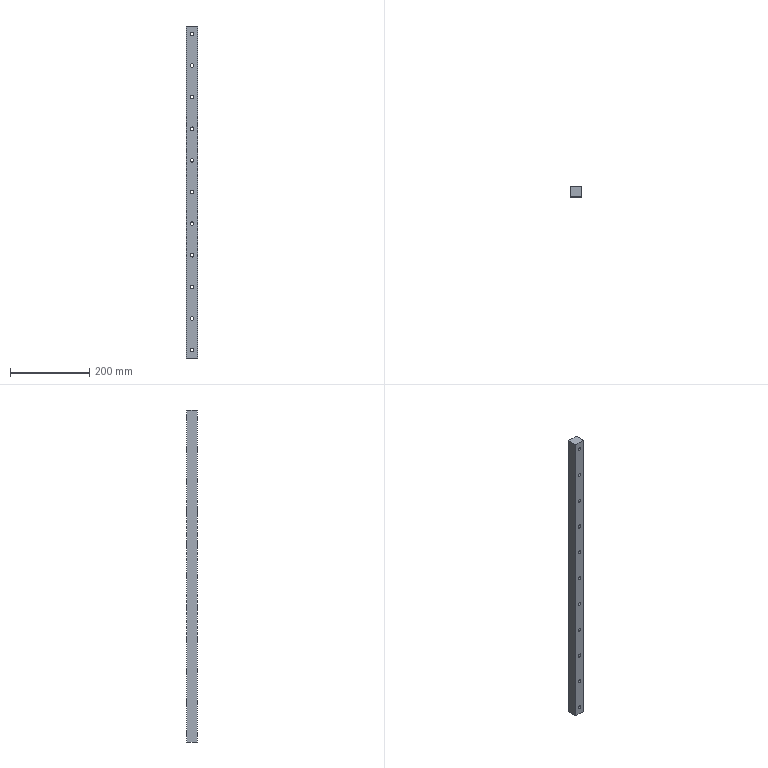Part | STEP file | P-008160^LM06S-05-03-02B_default | 1 solid | 61 faces | box 28 x 26 x 840 mm | volume 581403 mm3 | cylinder 44 | plane 17 | commonest cylinder face diameters 9 x22 14 x22